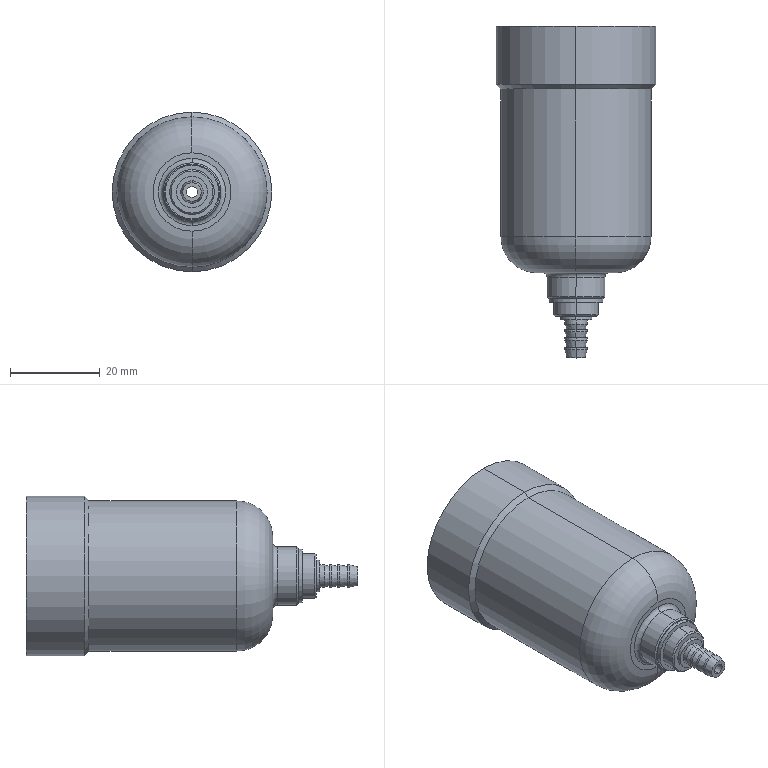Part | SolidWorks | features BaseBody 1 | 1 solid | 59 faces | box 35.6 x 74 x 35.6 mm | volume 13537 mm3 | cylinder 26 | cone 16 | plane 11 | torus 4 | spline 2 | commonest cylinder face diameters 5 x8 2.4 x2 7 x2 10 x2 12 x2 13 x2